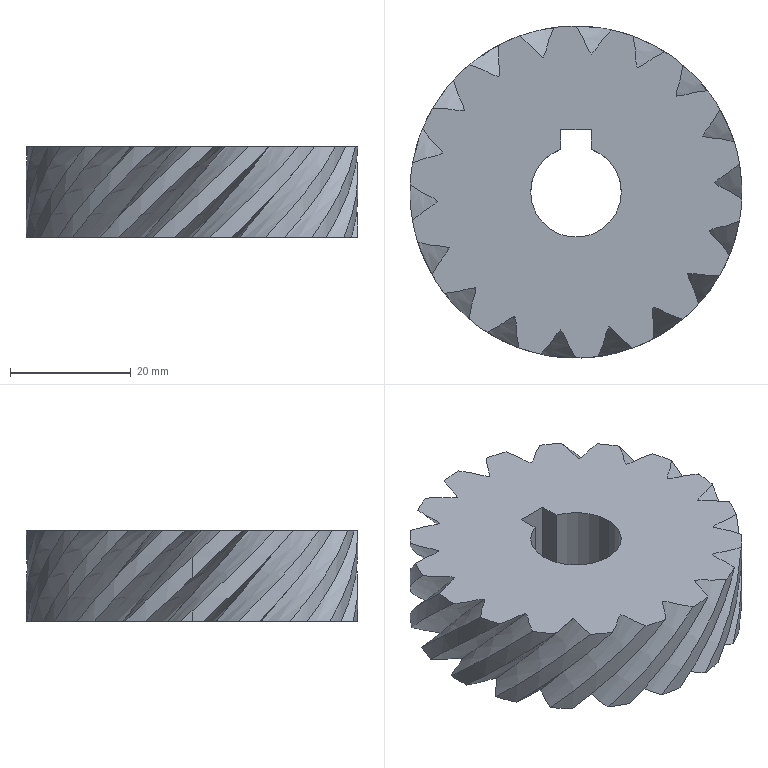Part | SolidWorks | features ICE 2, CirPattern 1, Extrusion 1, Helix 1, RefAxis 1, SweepCut 1 | 1 solid | 82 faces | box 54.912 x 54.912 x 15 mm | volume 29067 mm3 | spline 54 | cylinder 23 | plane 5 | commonest cylinder face diameters 54.912 x20 15 x3